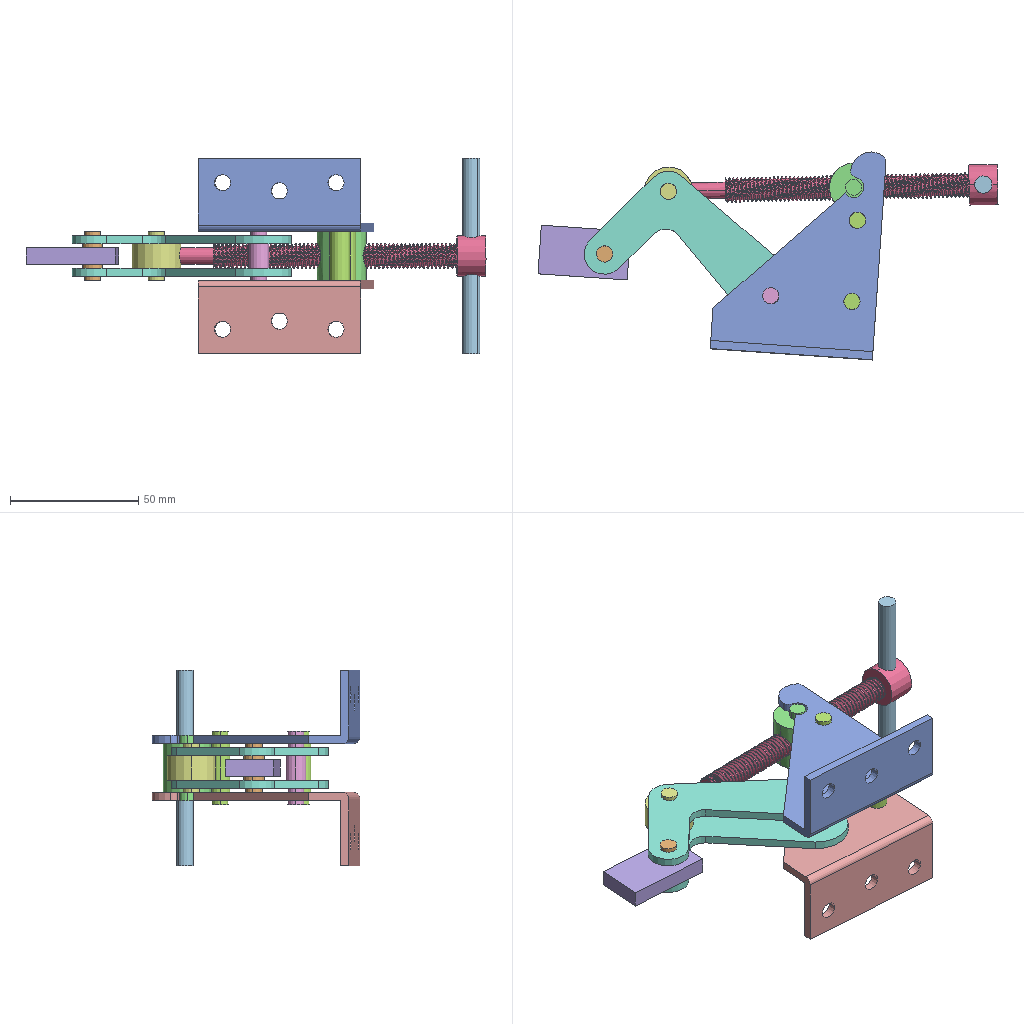Assembly | SolidWorks | 12 different items | 14 placed | box 180 x 81 x 76 mm
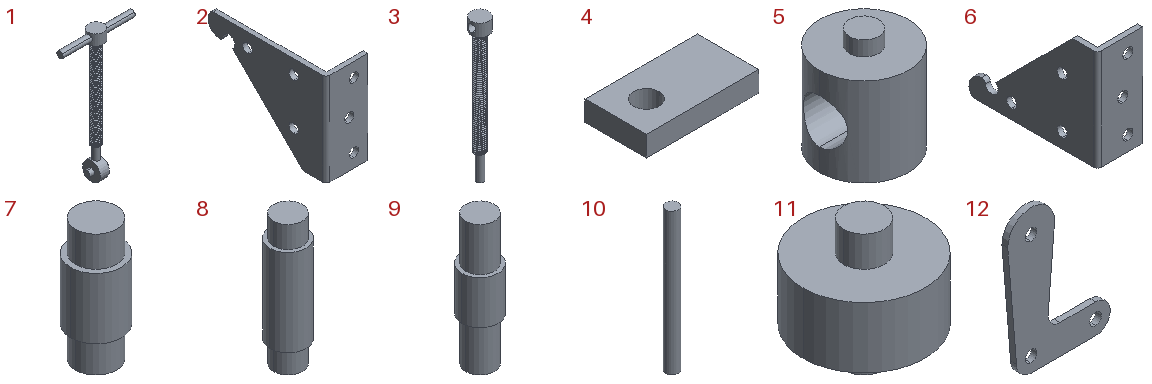Parts list (item | name | quantity | parent item | size | volume | features):
1 | (subassembly) | x1 | - | 76.2 x 19.05 x 138.125 mm | 13340 mm3 | -
2 | - | x1 | - | 28.575 x 80.975 x 63.5 mm | 14204 mm3 | features ICE 3, Extrusion 1
3 | - | x1 | in 1 | 15.875 x 15.875 x 128.6 mm | 7890 mm3 | features Helix 1, ICE 1, Revolution 1, SweepCut 1
4 | - | x1 | - | 34.925 x 19.05 x 6.35 mm | 3912 mm3 | features Extrusion 1
5 | - | x1 | - | 19.05 x 19.05 x 25.4 mm | 4317 mm3 | features ICE 2, Extrusion 1
6 | - | x1 | - | 28.575 x 80.975 x 63.5 mm | 14204 mm3 | features MirrorStock 1
7 | - | x1 | - | 7.925 x 7.925 x 19.05 mm | 771.469 mm3 | features Extrusion 1, ICE 1
8 | - | x2 | - | 7.925 x 7.925 x 28.575 mm | 1241 mm3 | features Extrusion 1, ICE 1
9 | - | x1 | - | 7.925 x 7.925 x 28.575 mm | 1073 mm3 | features Extrusion 1, ICE 1
10 | - | x1 | in 1 | 6.756 x 6.756 x 76.2 mm | 2732 mm3 | features Extrusion 1
11 | - | x1 | in 1 | 19.05 x 19.05 x 19.05 mm | 2719 mm3 | features ICE 3, Extrusion 1
12 | - | x2 | - | 55.575 x 3.175 x 77.8 mm | 6310 mm3 | features Extrusion 1
Mates (type | each side: item.copy, entity, surface, feature):
In the top assembly
Concentric | 2.1 face cylinder Boss-Extrude1 | 8.1 face cylinder Boss-Extrude2
Concentric | 6.1 face cylinder | 8.1 face cylinder Boss-Extrude2
Coincident | 6.1 face plane | 8.1 face plane Boss-Extrude1
Coincident | 2.1 face plane Boss-Extrude1 | 8.1 face plane Boss-Extrude1
Concentric | 2.1 face cylinder Boss-Extrude1 | 8.2 face cylinder Boss-Extrude2
Concentric | 6.1 face cylinder | 8.2 face cylinder Boss-Extrude2
Coincident | 6.1 face plane | 8.2 face plane Boss-Extrude1
Concentric | 2.1 face cylinder Boss-Extrude1 | 9.1 face cylinder Boss-Extrude2
Concentric | 6.1 face cylinder | 9.1 face cylinder Boss-Extrude2
Width | 8.2 face plane Boss-Extrude2 | 8.2 face plane Boss-Extrude2 | 9.1 face plane Boss-Extrude2 | 9.1 face plane Boss-Extrude2
Concentric | 9.1 face cylinder Boss-Extrude2 | 12.1 face cylinder Boss-Extrude1
Concentric | 9.1 face cylinder Boss-Extrude2 | 12.2 face cylinder Boss-Extrude1
Coincident | 9.1 face plane Boss-Extrude1 | 12.2 face plane Boss-Extrude1
Coincident | 9.1 face plane Boss-Extrude1 | 12.1 face plane Boss-Extrude1
Concentric | 12.2 face cylinder Boss-Extrude1 | 12.1 face cylinder Boss-Extrude1
Concentric | 12.2 face cylinder Boss-Extrude1 | 7.1 face cylinder Boss-Extrude2
Concentric | 12.1 face cylinder Boss-Extrude1 | 7.1 face cylinder Boss-Extrude2
Coincident | 12.1 face plane Boss-Extrude1 | 7.1 face plane Boss-Extrude1
Coincident | 12.2 face plane Boss-Extrude1 | 7.1 face plane Boss-Extrude1
Concentric | 7.1 face cylinder Boss-Extrude1 | 4.1 face cylinder Boss-Extrude1
Width | 4.1 face plane Boss-Extrude1 | 4.1 face plane Boss-Extrude1 | 12.2 face plane Boss-Extrude1 | 12.1 face plane Boss-Extrude1
Parallel | 2.1 face plane Boss-Extrude2 | 4.1 face plane Boss-Extrude1
Concentric | 2.1 face cylinder Boss-Extrude1 | 5.1 face cylinder Boss-Extrude2
Concentric | 6.1 face cylinder | 5.1 face cylinder Boss-Extrude2
Coincident | 6.1 face plane | 5.1 face plane Boss-Extrude2
Coincident | 2.1 face plane Boss-Extrude1 | 5.1 face plane Boss-Extrude2
Concentric | 12.2 face cylinder Boss-Extrude1 | 11.1 face cylinder Boss-Extrude3
Concentric | 12.1 face cylinder Boss-Extrude1 | 11.1 face cylinder Boss-Extrude2
Width | 12.2 face plane Boss-Extrude1 | 12.1 face plane Boss-Extrude1 | 11.1 face plane Boss-Extrude2 | 11.1 face plane Boss-Extrude3
Concentric | 5.1 face cylinder Cut-Extrude1 | 3.1 face cylinder Revolve2
In subassembly 1
Concentric | 3.2 face cylinder Cut-Extrude1 | 10.1 face cylinder Boss-Extrude1
Concentric | 3.2 face cylinder Revolve2 | 10.1 select_type:25
Coincident | 3.2 face plane Revolve2 | 11.2 face plane Cut-Extrude1
Concentric | 3.2 face cylinder Revolve2 | 11.2 face cylinder Cut-Extrude1